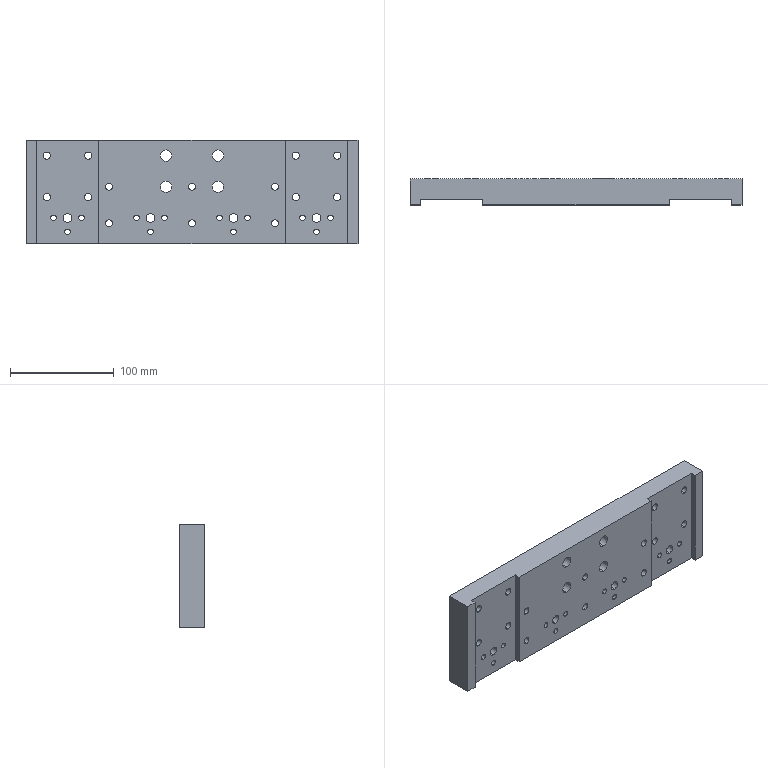Part | SolidWorks | features BaseBody 1 | 1 solid | 160 faces | box 320 x 25 x 100 mm | volume 683498 mm3 | cylinder 118 | plane 34 | cone 8 | commonest cylinder face diameters 5.2 x24 7 x16 13 x16 18 x16 6.8 x12 5 x10